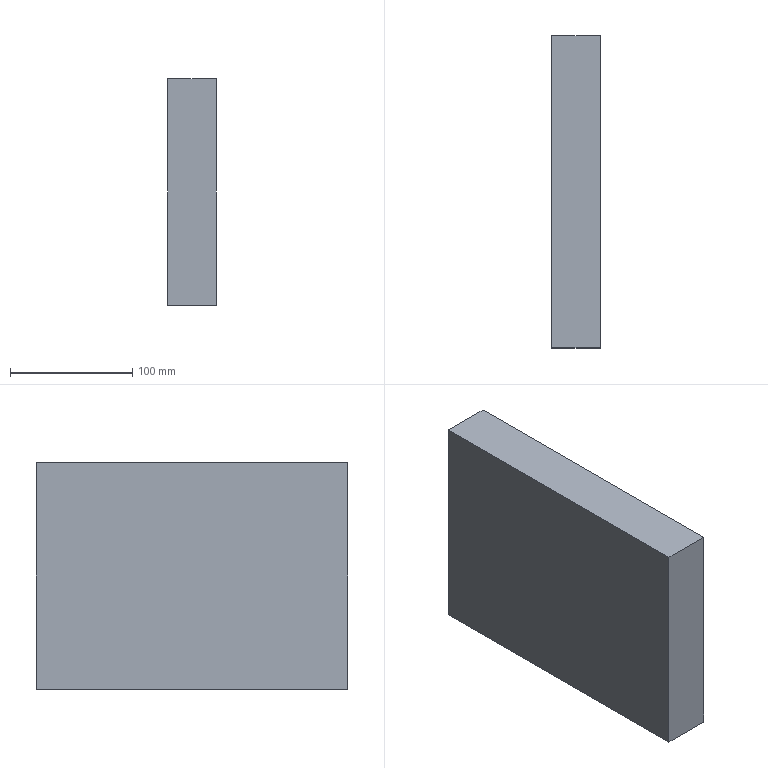Part | STEP file | 1 solid | 10 faces | box 40 x 255 x 185 mm | volume 1874377 mm3 | plane 6 | cylinder 2 | cone 2 | commonest cylinder face diameters 14 x2
STEP:
#1=CARTESIAN_POINT('',(-280.,-127.5,-292.));
#2=VERTEX_POINT('',#1);
#3=CARTESIAN_POINT('',(-280.,-127.5,-107.));
#4=VERTEX_POINT('',#3);
#5=CARTESIAN_POINT('',(-280.,-127.5,-107.));
#6=DIRECTION('',(0.,0.,1.));
#7=VECTOR('',#6,1.);
#8=LINE('',#5,#7);
#9=EDGE_CURVE('',#2,#4,#8,.T.);
#10=ORIENTED_EDGE('',*,*,#9,.T.);
#11=CARTESIAN_POINT('',(-280.,127.5,-107.));
#12=VERTEX_POINT('',#11);
#13=CARTESIAN_POINT('',(-280.,-1.,-107.));
#14=DIRECTION('',(0.,-1.,0.));
#15=VECTOR('',#14,1.);
#16=LINE('',#13,#15);
#17=EDGE_CURVE('',#12,#4,#16,.T.);
#18=ORIENTED_EDGE('',*,*,#17,.F.);
#19=CARTESIAN_POINT('',(-280.,127.5,-292.));
#20=VERTEX_POINT('',#19);
#21=CARTESIAN_POINT('',(-280.,127.5,-107.));
#22=DIRECTION('',(0.,0.,1.));
#23=VECTOR('',#22,1.);
#24=LINE('',#21,#23);
#25=EDGE_CURVE('',#20,#12,#24,.T.);
#26=ORIENTED_EDGE('',*,*,#25,.F.);
#27=CARTESIAN_POINT('',(-280.,-1.,-292.));
#28=DIRECTION('',(0.,-1.,0.));
#29=VECTOR('',#28,1.);
#30=LINE('',#27,#29);
#31=EDGE_CURVE('',#20,#2,#30,.T.);
#32=ORIENTED_EDGE('',*,*,#31,.T.);
#33=EDGE_LOOP('',(#10,#18,#26,#32));
#34=FACE_OUTER_BOUND('',#33,.T.);
#35=CARTESIAN_POINT('',(-280.,-1.,-107.));
#36=DIRECTION('',(-1.,0.,0.));
#37=DIRECTION('',(0.,-1.,0.));
#38=AXIS2_PLACEMENT_3D('',#35,#36,#37);
#39=PLANE('',#38);
#40=ADVANCED_FACE('',(#34),#39,.T.);
#41=ORIENTED_EDGE('',*,*,#25,.T.);
#42=CARTESIAN_POINT('',(-240.,127.5,-107.));
#43=VERTEX_POINT('',#42);
#44=CARTESIAN_POINT('',(178.5,127.5,-107.));
#45=DIRECTION('',(-1.,0.,0.));
#46=VECTOR('',#45,1.);
#47=LINE('',#44,#46);
#48=EDGE_CURVE('',#43,#12,#47,.T.);
#49=ORIENTED_EDGE('',*,*,#48,.F.);
#50=CARTESIAN_POINT('',(-240.,127.5,-292.));
#51=VERTEX_POINT('',#50);
#52=CARTESIAN_POINT('',(-240.,127.5,-107.));
#53=DIRECTION('',(0.,0.,1.));
#54=VECTOR('',#53,1.);
#55=LINE('',#52,#54);
#56=EDGE_CURVE('',#51,#43,#55,.T.);
#57=ORIENTED_EDGE('',*,*,#56,.F.);
#58=CARTESIAN_POINT('',(178.5,127.5,-292.));
#59=DIRECTION('',(-1.,0.,0.));
#60=VECTOR('',#59,1.);
#61=LINE('',#58,#60);
#62=EDGE_CURVE('',#51,#20,#61,.T.);
#63=ORIENTED_EDGE('',*,*,#62,.T.);
#64=EDGE_LOOP('',(#41,#49,#57,#63));
#65=FACE_OUTER_BOUND('',#64,.T.);
#66=CARTESIAN_POINT('',(178.5,127.5,-107.));
#67=DIRECTION('',(0.,1.,0.));
#68=DIRECTION('',(-1.,0.,0.));
#69=AXIS2_PLACEMENT_3D('',#66,#67,#68);
#70=PLANE('',#69);
#71=ADVANCED_FACE('',(#65),#70,.T.);
#72=ORIENTED_EDGE('',*,*,#56,.T.);
#73=CARTESIAN_POINT('',(-240.,-127.5,-107.));
#74=VERTEX_POINT('',#73);
#75=CARTESIAN_POINT('',(-240.,-1.,-107.));
#76=DIRECTION('',(0.,1.,0.));
#77=VECTOR('',#76,1.);
#78=LINE('',#75,#77);
#79=EDGE_CURVE('',#74,#43,#78,.T.);
#80=ORIENTED_EDGE('',*,*,#79,.F.);
#81=CARTESIAN_POINT('',(-240.,-127.5,-292.));
#82=VERTEX_POINT('',#81);
#83=CARTESIAN_POINT('',(-240.,-127.5,-107.));
#84=DIRECTION('',(0.,0.,1.));
#85=VECTOR('',#84,1.);
#86=LINE('',#83,#85);
#87=EDGE_CURVE('',#82,#74,#86,.T.);
#88=ORIENTED_EDGE('',*,*,#87,.F.);
#89=CARTESIAN_POINT('',(-240.,-1.,-292.));
#90=DIRECTION('',(0.,1.,0.));
#91=VECTOR('',#90,1.);
#92=LINE('',#89,#91);
#93=EDGE_CURVE('',#82,#51,#92,.T.);
#94=ORIENTED_EDGE('',*,*,#93,.T.);
#95=EDGE_LOOP('',(#72,#80,#88,#94));
#96=FACE_OUTER_BOUND('',#95,.T.);
#97=CARTESIAN_POINT('',(-240.,-1.,-107.));
#98=DIRECTION('',(1.,0.,0.));
#99=DIRECTION('',(0.,1.,0.));
#100=AXIS2_PLACEMENT_3D('',#97,#98,#99);
#101=PLANE('',#100);
#102=ADVANCED_FACE('',(#96),#101,.T.);
#103=CARTESIAN_POINT('',(178.5,-127.5,-292.));
#104=DIRECTION('',(1.,0.,0.));
#105=VECTOR('',#104,1.);
#106=LINE('',#103,#105);
#107=EDGE_CURVE('',#2,#82,#106,.T.);
#108=ORIENTED_EDGE('',*,*,#107,.T.);
#109=ORIENTED_EDGE('',*,*,#87,.T.);
#110=CARTESIAN_POINT('',(178.5,-127.5,-107.));
#111=DIRECTION('',(1.,0.,0.));
#112=VECTOR('',#111,1.);
#113=LINE('',#110,#112);
#114=EDGE_CURVE('',#4,#74,#113,.T.);
#115=ORIENTED_EDGE('',*,*,#114,.F.);
#116=ORIENTED_EDGE('',*,*,#9,.F.);
#117=EDGE_LOOP('',(#108,#109,#115,#116));
#118=FACE_OUTER_BOUND('',#117,.T.);
#119=CARTESIAN_POINT('',(178.5,-127.5,-107.));
#120=DIRECTION('',(0.,-1.,0.));
#121=DIRECTION('',(1.,0.,0.));
#122=AXIS2_PLACEMENT_3D('',#119,#120,#121);
#123=PLANE('',#122);
#124=ADVANCED_FACE('',(#118),#123,.T.);
#125=ORIENTED_EDGE('',*,*,#79,.T.);
#126=ORIENTED_EDGE('',*,*,#48,.T.);
#127=ORIENTED_EDGE('',*,*,#17,.T.);
#128=ORIENTED_EDGE('',*,*,#114,.T.);
#129=EDGE_LOOP('',(#125,#126,#127,#128));
#130=FACE_OUTER_BOUND('',#129,.T.);
#131=CARTESIAN_POINT('',(178.5,-1.,-107.));
#132=DIRECTION('',(0.,0.,1.));
#133=DIRECTION('',(1.,0.,0.));
#134=AXIS2_PLACEMENT_3D('',#131,#132,#133);
#135=PLANE('',#134);
#136=ADVANCED_FACE('',(#130),#135,.T.);
#137=ORIENTED_EDGE('',*,*,#93,.F.);
#138=ORIENTED_EDGE('',*,*,#107,.F.);
#139=ORIENTED_EDGE('',*,*,#31,.F.);
#140=ORIENTED_EDGE('',*,*,#62,.F.);
#141=EDGE_LOOP('',(#137,#138,#139,#140));
#142=FACE_BOUND('',#141,.T.);
#143=CARTESIAN_POINT('',(-253.,102.5,-292.));
#144=VERTEX_POINT('',#143);
#145=CARTESIAN_POINT('',(-260.,102.5,-292.));
#146=DIRECTION('',(0.,0.,1.));
#147=DIRECTION('',(1.,0.,0.));
#148=AXIS2_PLACEMENT_3D('',#145,#146,#147);
#149=CIRCLE('',#148,7.);
#150=EDGE_CURVE('',#144,#144,#149,.T.);
#151=ORIENTED_EDGE('',*,*,#150,.T.);
#152=EDGE_LOOP('',(#151));
#153=FACE_BOUND('',#152,.T.);
#154=CARTESIAN_POINT('',(-253.,-102.5,-292.));
#155=VERTEX_POINT('',#154);
#156=CARTESIAN_POINT('',(-260.,-102.5,-292.));
#157=DIRECTION('',(0.,0.,-1.));
#158=DIRECTION('',(1.,0.,0.));
#159=AXIS2_PLACEMENT_3D('',#156,#157,#158);
#160=CIRCLE('',#159,7.);
#161=EDGE_CURVE('',#155,#155,#160,.T.);
#162=ORIENTED_EDGE('',*,*,#161,.F.);
#163=EDGE_LOOP('',(#162));
#164=FACE_BOUND('',#163,.T.);
#165=CARTESIAN_POINT('',(168.5,-1.,-292.));
#166=DIRECTION('',(0.,0.,-1.));
#167=DIRECTION('',(1.,0.,0.));
#168=AXIS2_PLACEMENT_3D('',#165,#166,#167);
#169=PLANE('',#168);
#170=ADVANCED_FACE('',(#142,#153,#164),#169,.T.);
#171=CARTESIAN_POINT('',(-267.,102.5,-252.));
#172=VERTEX_POINT('',#171);
#173=CARTESIAN_POINT('',(-260.,102.5,-252.));
#174=DIRECTION('',(0.,0.,-1.));
#175=DIRECTION('',(-1.,0.,0.));
#176=AXIS2_PLACEMENT_3D('',#173,#174,#175);
#177=CIRCLE('',#176,7.);
#178=EDGE_CURVE('',#172,#172,#177,.T.);
#179=ORIENTED_EDGE('',*,*,#178,.F.);
#180=EDGE_LOOP('',(#179));
#181=FACE_BOUND('',#180,.T.);
#182=ORIENTED_EDGE('',*,*,#150,.F.);
#183=EDGE_LOOP('',(#182));
#184=FACE_BOUND('',#183,.T.);
#185=CARTESIAN_POINT('',(-260.,102.5,-292.));
#186=DIRECTION('',(0.,0.,1.));
#187=DIRECTION('',(-1.,0.,0.));
#188=AXIS2_PLACEMENT_3D('',#185,#186,#187);
#189=CYLINDRICAL_SURFACE('',#188,7.);
#190=ADVANCED_FACE('',(#181,#184),#189,.F.);
#191=ORIENTED_EDGE('',*,*,#178,.T.);
#192=EDGE_LOOP('',(#191));
#193=FACE_BOUND('',#192,.T.);
#194=CARTESIAN_POINT('',(-260.,102.5,-249.));
#195=VERTEX_POINT('',#194);
#196=VERTEX_LOOP('',#195);
#197=FACE_BOUND('',#196,.T.);
#198=CARTESIAN_POINT('',(-260.,102.5,-249.));
#199=DIRECTION('',(0.,0.,-1.));
#200=DIRECTION('',(-1.,0.,0.));
#201=AXIS2_PLACEMENT_3D('',#198,#199,#200);
#202=CONICAL_SURFACE('',#201,0.,66.801);
#203=ADVANCED_FACE('',(#193,#197),#202,.F.);
#204=CARTESIAN_POINT('',(-267.,-102.5,-252.));
#205=VERTEX_POINT('',#204);
#206=CARTESIAN_POINT('',(-260.,-102.5,-252.));
#207=DIRECTION('',(0.,0.,1.));
#208=DIRECTION('',(-1.,0.,0.));
#209=AXIS2_PLACEMENT_3D('',#206,#207,#208);
#210=CIRCLE('',#209,7.);
#211=EDGE_CURVE('',#205,#205,#210,.T.);
#212=ORIENTED_EDGE('',*,*,#211,.T.);
#213=EDGE_LOOP('',(#212));
#214=FACE_BOUND('',#213,.T.);
#215=ORIENTED_EDGE('',*,*,#161,.T.);
#216=EDGE_LOOP('',(#215));
#217=FACE_BOUND('',#216,.T.);
#218=CARTESIAN_POINT('',(-260.,-102.5,-292.));
#219=DIRECTION('',(0.,0.,1.));
#220=DIRECTION('',(-1.,0.,0.));
#221=AXIS2_PLACEMENT_3D('',#218,#219,#220);
#222=CYLINDRICAL_SURFACE('',#221,7.);
#223=ADVANCED_FACE('',(#214,#217),#222,.F.);
#224=ORIENTED_EDGE('',*,*,#211,.F.);
#225=EDGE_LOOP('',(#224));
#226=FACE_BOUND('',#225,.T.);
#227=CARTESIAN_POINT('',(-260.,-102.5,-249.));
#228=VERTEX_POINT('',#227);
#229=VERTEX_LOOP('',#228);
#230=FACE_BOUND('',#229,.T.);
#231=CARTESIAN_POINT('',(-260.,-102.5,-249.));
#232=DIRECTION('',(0.,0.,-1.));
#233=DIRECTION('',(-1.,0.,0.));
#234=AXIS2_PLACEMENT_3D('',#231,#232,#233);
#235=CONICAL_SURFACE('',#234,0.,66.801);
#236=ADVANCED_FACE('',(#226,#230),#235,.F.);
#237=CLOSED_SHELL('',(#40,#71,#102,#124,#136,#170,#190,#203,#223,#236));
#238=MANIFOLD_SOLID_BREP('',#237);
#239=(LENGTH_UNIT()NAMED_UNIT(*)SI_UNIT(.MILLI.,.METRE.));
#240=UNCERTAINTY_MEASURE_WITH_UNIT(LENGTH_MEASURE(0.00002),#239,'','');
#241=(NAMED_UNIT(*)PLANE_ANGLE_UNIT()SI_UNIT($,.RADIAN.));
#242=PLANE_ANGLE_MEASURE_WITH_UNIT(PLANE_ANGLE_MEASURE(0.01745),#241);
#243=DIMENSIONAL_EXPONENTS(0.,0.,0.,0.,0.,0.,0.);
#244=(CONVERSION_BASED_UNIT('DEGREE',#242)NAMED_UNIT(#243)PLANE_ANGLE_UNIT());
#245=(NAMED_UNIT(*)SI_UNIT($,.STERADIAN.)SOLID_ANGLE_UNIT());
#246=(GEOMETRIC_REPRESENTATION_CONTEXT(3)GLOBAL_UNCERTAINTY_ASSIGNED_CONTEXT((#240))GLOBAL_UNIT_ASSIGNED_CONTEXT((#239,#244,#245))REPRESENTATION_CONTEXT('',''));
#247=ADVANCED_BREP_SHAPE_REPRESENTATION('',(#238),#246);